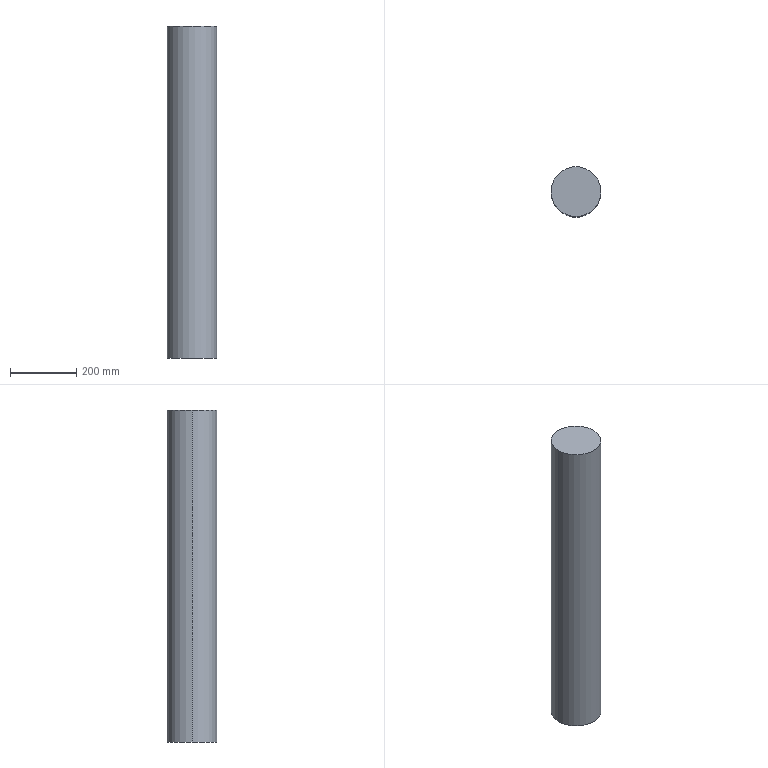Part | SolidWorks | features Extrusion 1 | 1 solid | 4 faces | box 150 x 150 x 1000 mm | volume 17671459 mm3 | cylinder 2 | plane 2 | commonest cylinder face diameters 150 x2
STEP:
#1=CARTESIAN_POINT('',(75.,0.,1000.));
#2=VERTEX_POINT('',#1);
#3=CARTESIAN_POINT('',(-75.,0.,1000.));
#4=VERTEX_POINT('',#3);
#5=CARTESIAN_POINT('',(0.,0.,1000.));
#6=DIRECTION('',(0.,0.,1.));
#7=DIRECTION('',(1.,0.,0.));
#8=AXIS2_PLACEMENT_3D('',#5,#6,#7);
#9=CIRCLE('',#8,75.);
#10=EDGE_CURVE('',#2,#4,#9,.T.);
#11=ORIENTED_EDGE('',*,*,#10,.F.);
#12=CARTESIAN_POINT('',(75.,0.,0.));
#13=VERTEX_POINT('',#12);
#14=CARTESIAN_POINT('',(75.,0.,1000.));
#15=DIRECTION('',(0.,0.,-1.));
#16=VECTOR('',#15,1000.);
#17=LINE('',#14,#16);
#18=EDGE_CURVE('',#2,#13,#17,.T.);
#19=ORIENTED_EDGE('',*,*,#18,.T.);
#20=CARTESIAN_POINT('',(-75.,0.,0.));
#21=VERTEX_POINT('',#20);
#22=CARTESIAN_POINT('',(0.,0.,0.));
#23=DIRECTION('',(0.,0.,1.));
#24=DIRECTION('',(1.,0.,0.));
#25=AXIS2_PLACEMENT_3D('',#22,#23,#24);
#26=CIRCLE('',#25,75.);
#27=EDGE_CURVE('',#13,#21,#26,.T.);
#28=ORIENTED_EDGE('',*,*,#27,.T.);
#29=CARTESIAN_POINT('',(-75.,0.,1000.));
#30=DIRECTION('',(0.,0.,-1.));
#31=VECTOR('',#30,1000.);
#32=LINE('',#29,#31);
#33=EDGE_CURVE('',#4,#21,#32,.T.);
#34=ORIENTED_EDGE('',*,*,#33,.F.);
#35=EDGE_LOOP('',(#11,#19,#28,#34));
#36=FACE_OUTER_BOUND('',#35,.T.);
#37=CARTESIAN_POINT('',(0.,0.,1000.));
#38=DIRECTION('',(0.,0.,-1.));
#39=DIRECTION('',(-1.,0.,0.));
#40=AXIS2_PLACEMENT_3D('',#37,#38,#39);
#41=CYLINDRICAL_SURFACE('',#40,75.);
#42=ADVANCED_FACE('',(#36),#41,.T.);
#43=ORIENTED_EDGE('',*,*,#18,.F.);
#44=CARTESIAN_POINT('',(0.,0.,1000.));
#45=DIRECTION('',(0.,0.,1.));
#46=DIRECTION('',(1.,0.,0.));
#47=AXIS2_PLACEMENT_3D('',#44,#45,#46);
#48=CIRCLE('',#47,75.);
#49=EDGE_CURVE('',#4,#2,#48,.T.);
#50=ORIENTED_EDGE('',*,*,#49,.F.);
#51=ORIENTED_EDGE('',*,*,#33,.T.);
#52=CARTESIAN_POINT('',(0.,0.,0.));
#53=DIRECTION('',(0.,0.,1.));
#54=DIRECTION('',(1.,0.,0.));
#55=AXIS2_PLACEMENT_3D('',#52,#53,#54);
#56=CIRCLE('',#55,75.);
#57=EDGE_CURVE('',#21,#13,#56,.T.);
#58=ORIENTED_EDGE('',*,*,#57,.T.);
#59=EDGE_LOOP('',(#43,#50,#51,#58));
#60=FACE_OUTER_BOUND('',#59,.T.);
#61=CARTESIAN_POINT('',(0.,0.,1000.));
#62=DIRECTION('',(0.,0.,-1.));
#63=DIRECTION('',(-1.,0.,0.));
#64=AXIS2_PLACEMENT_3D('',#61,#62,#63);
#65=CYLINDRICAL_SURFACE('',#64,75.);
#66=ADVANCED_FACE('',(#60),#65,.T.);
#67=ORIENTED_EDGE('',*,*,#49,.T.);
#68=ORIENTED_EDGE('',*,*,#10,.T.);
#69=EDGE_LOOP('',(#67,#68));
#70=FACE_OUTER_BOUND('',#69,.T.);
#71=CARTESIAN_POINT('',(0.,0.,1000.));
#72=DIRECTION('',(0.,0.,1.));
#73=DIRECTION('',(1.,0.,0.));
#74=AXIS2_PLACEMENT_3D('',#71,#72,#73);
#75=PLANE('',#74);
#76=ADVANCED_FACE('',(#70),#75,.T.);
#77=ORIENTED_EDGE('',*,*,#57,.F.);
#78=ORIENTED_EDGE('',*,*,#27,.F.);
#79=EDGE_LOOP('',(#77,#78));
#80=FACE_OUTER_BOUND('',#79,.T.);
#81=CARTESIAN_POINT('',(0.,0.,0.));
#82=DIRECTION('',(0.,0.,1.));
#83=DIRECTION('',(1.,0.,0.));
#84=AXIS2_PLACEMENT_3D('',#81,#82,#83);
#85=PLANE('',#84);
#86=ADVANCED_FACE('',(#80),#85,.F.);
#87=CLOSED_SHELL('',(#42,#66,#76,#86));
#88=MANIFOLD_SOLID_BREP('',#87);
#89=CARTESIAN_POINT('',(0.,0.,0.));
#90=DIRECTION('',(0.,0.,1.));
#91=DIRECTION('',(1.,0.,0.));
#92=AXIS2_PLACEMENT_3D('',#89,#90,#91);
#93=(LENGTH_UNIT()NAMED_UNIT(*)SI_UNIT(.MILLI.,.METRE.));
#94=UNCERTAINTY_MEASURE_WITH_UNIT(LENGTH_MEASURE(0.00001),#93,'','');
#95=(NAMED_UNIT(*)PLANE_ANGLE_UNIT()SI_UNIT($,.RADIAN.));
#96=(NAMED_UNIT(*)SI_UNIT($,.STERADIAN.)SOLID_ANGLE_UNIT());
#97=(GEOMETRIC_REPRESENTATION_CONTEXT(3)GLOBAL_UNCERTAINTY_ASSIGNED_CONTEXT((#94))GLOBAL_UNIT_ASSIGNED_CONTEXT((#93,#95,#96))REPRESENTATION_CONTEXT('',''));
#98=ADVANCED_BREP_SHAPE_REPRESENTATION('',(#88,#92),#97);